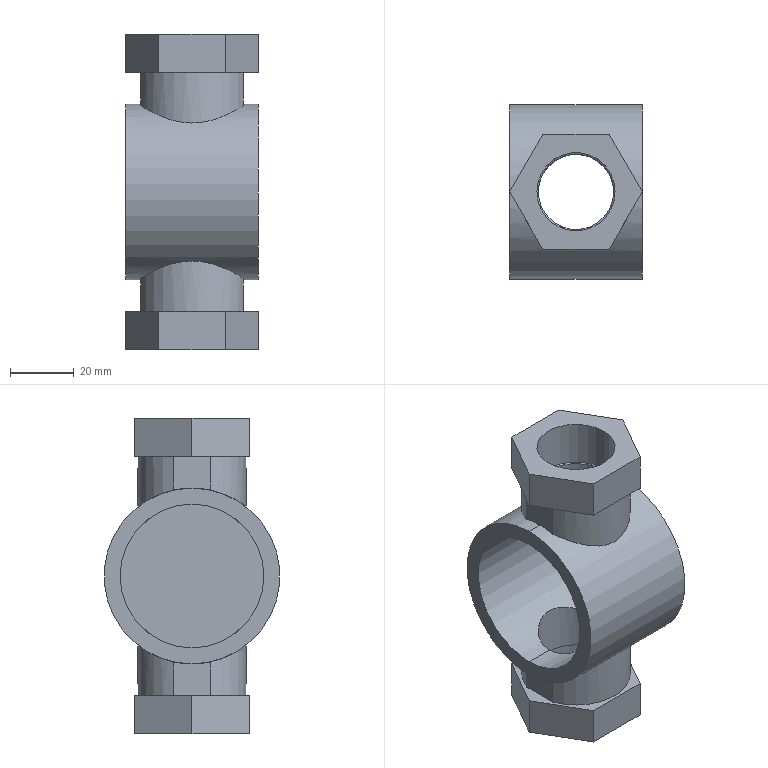Part | SolidWorks | features ICE 5, HoleWzd 2, Extrusion 1, MirrorPattern 1 | 1 solid | 43 faces | box 41.569 x 55 x 99 mm | volume 62530 mm3 | plane 23 | cylinder 16 | cone 4 | commonest cylinder face diameters 23.65 x4 24.5 x4 34 x4 45 x2 55 x2